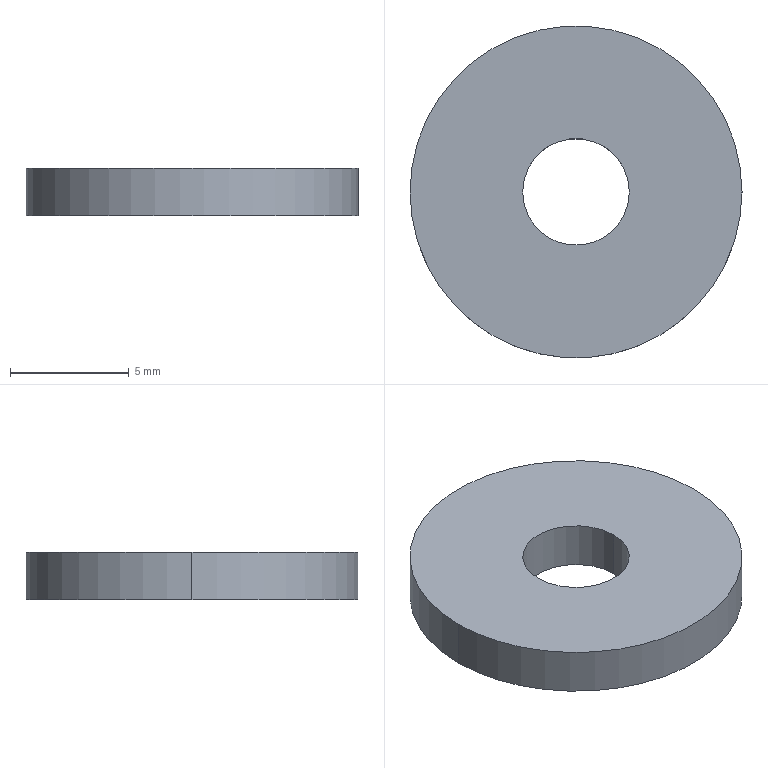Part | SolidWorks | features Extrusion 1 | 1 solid | 6 faces | box 14 x 14 x 2 mm | volume 276.067 mm3 | cylinder 4 | plane 2 | commonest cylinder face diameters 4.5 x2 14 x2
STEP:
#1=CARTESIAN_POINT('',(-2.25,0.,2.));
#2=VERTEX_POINT('',#1);
#3=CARTESIAN_POINT('',(2.25,0.,2.));
#4=VERTEX_POINT('',#3);
#5=CARTESIAN_POINT('',(0.,0.,2.));
#6=DIRECTION('',(0.,0.,1.));
#7=DIRECTION('',(1.,0.,0.));
#8=AXIS2_PLACEMENT_3D('',#5,#6,#7);
#9=CIRCLE('',#8,2.25);
#10=EDGE_CURVE('',#2,#4,#9,.T.);
#11=ORIENTED_EDGE('',*,*,#10,.T.);
#12=CARTESIAN_POINT('',(2.25,0.,0.));
#13=VERTEX_POINT('',#12);
#14=CARTESIAN_POINT('',(2.25,0.,2.));
#15=DIRECTION('',(0.,0.,-1.));
#16=VECTOR('',#15,1000.);
#17=LINE('',#14,#16);
#18=EDGE_CURVE('',#4,#13,#17,.T.);
#19=ORIENTED_EDGE('',*,*,#18,.T.);
#20=CARTESIAN_POINT('',(-2.25,0.,0.));
#21=VERTEX_POINT('',#20);
#22=CARTESIAN_POINT('',(0.,0.,0.));
#23=DIRECTION('',(0.,0.,1.));
#24=DIRECTION('',(1.,0.,0.));
#25=AXIS2_PLACEMENT_3D('',#22,#23,#24);
#26=CIRCLE('',#25,2.25);
#27=EDGE_CURVE('',#21,#13,#26,.T.);
#28=ORIENTED_EDGE('',*,*,#27,.F.);
#29=CARTESIAN_POINT('',(-2.25,0.,2.));
#30=DIRECTION('',(0.,0.,-1.));
#31=VECTOR('',#30,1000.);
#32=LINE('',#29,#31);
#33=EDGE_CURVE('',#2,#21,#32,.T.);
#34=ORIENTED_EDGE('',*,*,#33,.F.);
#35=EDGE_LOOP('',(#11,#19,#28,#34));
#36=FACE_OUTER_BOUND('',#35,.T.);
#37=CARTESIAN_POINT('',(0.,0.,2.));
#38=DIRECTION('',(0.,0.,-1.));
#39=DIRECTION('',(-1.,0.,0.));
#40=AXIS2_PLACEMENT_3D('',#37,#38,#39);
#41=CYLINDRICAL_SURFACE('',#40,2.25);
#42=ADVANCED_FACE('',(#36),#41,.F.);
#43=CARTESIAN_POINT('',(7.,0.,2.));
#44=VERTEX_POINT('',#43);
#45=CARTESIAN_POINT('',(-7.,0.,2.));
#46=VERTEX_POINT('',#45);
#47=CARTESIAN_POINT('',(0.,0.,2.));
#48=DIRECTION('',(0.,0.,1.));
#49=DIRECTION('',(1.,0.,0.));
#50=AXIS2_PLACEMENT_3D('',#47,#48,#49);
#51=CIRCLE('',#50,7.);
#52=EDGE_CURVE('',#44,#46,#51,.T.);
#53=ORIENTED_EDGE('',*,*,#52,.F.);
#54=CARTESIAN_POINT('',(7.,0.,0.));
#55=VERTEX_POINT('',#54);
#56=CARTESIAN_POINT('',(7.,0.,2.));
#57=DIRECTION('',(0.,0.,-1.));
#58=VECTOR('',#57,1000.);
#59=LINE('',#56,#58);
#60=EDGE_CURVE('',#44,#55,#59,.T.);
#61=ORIENTED_EDGE('',*,*,#60,.T.);
#62=CARTESIAN_POINT('',(-7.,0.,0.));
#63=VERTEX_POINT('',#62);
#64=CARTESIAN_POINT('',(0.,0.,0.));
#65=DIRECTION('',(0.,0.,1.));
#66=DIRECTION('',(1.,0.,0.));
#67=AXIS2_PLACEMENT_3D('',#64,#65,#66);
#68=CIRCLE('',#67,7.);
#69=EDGE_CURVE('',#55,#63,#68,.T.);
#70=ORIENTED_EDGE('',*,*,#69,.T.);
#71=CARTESIAN_POINT('',(-7.,0.,2.));
#72=DIRECTION('',(0.,0.,-1.));
#73=VECTOR('',#72,1000.);
#74=LINE('',#71,#73);
#75=EDGE_CURVE('',#46,#63,#74,.T.);
#76=ORIENTED_EDGE('',*,*,#75,.F.);
#77=EDGE_LOOP('',(#53,#61,#70,#76));
#78=FACE_OUTER_BOUND('',#77,.T.);
#79=CARTESIAN_POINT('',(0.,0.,2.));
#80=DIRECTION('',(0.,0.,-1.));
#81=DIRECTION('',(-1.,0.,0.));
#82=AXIS2_PLACEMENT_3D('',#79,#80,#81);
#83=CYLINDRICAL_SURFACE('',#82,7.);
#84=ADVANCED_FACE('',(#78),#83,.T.);
#85=CARTESIAN_POINT('',(0.,0.,2.));
#86=DIRECTION('',(0.,0.,1.));
#87=DIRECTION('',(1.,0.,0.));
#88=AXIS2_PLACEMENT_3D('',#85,#86,#87);
#89=CIRCLE('',#88,7.);
#90=EDGE_CURVE('',#46,#44,#89,.T.);
#91=ORIENTED_EDGE('',*,*,#90,.T.);
#92=ORIENTED_EDGE('',*,*,#52,.T.);
#93=EDGE_LOOP('',(#91,#92));
#94=FACE_OUTER_BOUND('',#93,.T.);
#95=ORIENTED_EDGE('',*,*,#10,.F.);
#96=CARTESIAN_POINT('',(0.,0.,2.));
#97=DIRECTION('',(0.,0.,1.));
#98=DIRECTION('',(1.,0.,0.));
#99=AXIS2_PLACEMENT_3D('',#96,#97,#98);
#100=CIRCLE('',#99,2.25);
#101=EDGE_CURVE('',#4,#2,#100,.T.);
#102=ORIENTED_EDGE('',*,*,#101,.F.);
#103=EDGE_LOOP('',(#95,#102));
#104=FACE_BOUND('',#103,.T.);
#105=CARTESIAN_POINT('',(0.,0.,2.));
#106=DIRECTION('',(0.,0.,1.));
#107=DIRECTION('',(1.,0.,0.));
#108=AXIS2_PLACEMENT_3D('',#105,#106,#107);
#109=PLANE('',#108);
#110=ADVANCED_FACE('',(#94,#104),#109,.T.);
#111=CARTESIAN_POINT('',(0.,0.,0.));
#112=DIRECTION('',(0.,0.,1.));
#113=DIRECTION('',(1.,0.,0.));
#114=AXIS2_PLACEMENT_3D('',#111,#112,#113);
#115=CIRCLE('',#114,7.);
#116=EDGE_CURVE('',#63,#55,#115,.T.);
#117=ORIENTED_EDGE('',*,*,#116,.F.);
#118=ORIENTED_EDGE('',*,*,#69,.F.);
#119=EDGE_LOOP('',(#117,#118));
#120=FACE_OUTER_BOUND('',#119,.T.);
#121=ORIENTED_EDGE('',*,*,#27,.T.);
#122=CARTESIAN_POINT('',(0.,0.,0.));
#123=DIRECTION('',(0.,0.,1.));
#124=DIRECTION('',(1.,0.,0.));
#125=AXIS2_PLACEMENT_3D('',#122,#123,#124);
#126=CIRCLE('',#125,2.25);
#127=EDGE_CURVE('',#13,#21,#126,.T.);
#128=ORIENTED_EDGE('',*,*,#127,.T.);
#129=EDGE_LOOP('',(#121,#128));
#130=FACE_BOUND('',#129,.T.);
#131=CARTESIAN_POINT('',(0.,0.,0.));
#132=DIRECTION('',(0.,0.,1.));
#133=DIRECTION('',(1.,0.,0.));
#134=AXIS2_PLACEMENT_3D('',#131,#132,#133);
#135=PLANE('',#134);
#136=ADVANCED_FACE('',(#120,#130),#135,.F.);
#137=ORIENTED_EDGE('',*,*,#60,.F.);
#138=ORIENTED_EDGE('',*,*,#90,.F.);
#139=ORIENTED_EDGE('',*,*,#75,.T.);
#140=ORIENTED_EDGE('',*,*,#116,.T.);
#141=EDGE_LOOP('',(#137,#138,#139,#140));
#142=FACE_OUTER_BOUND('',#141,.T.);
#143=CARTESIAN_POINT('',(0.,0.,2.));
#144=DIRECTION('',(0.,0.,-1.));
#145=DIRECTION('',(-1.,0.,0.));
#146=AXIS2_PLACEMENT_3D('',#143,#144,#145);
#147=CYLINDRICAL_SURFACE('',#146,7.);
#148=ADVANCED_FACE('',(#142),#147,.T.);
#149=ORIENTED_EDGE('',*,*,#18,.F.);
#150=ORIENTED_EDGE('',*,*,#101,.T.);
#151=ORIENTED_EDGE('',*,*,#33,.T.);
#152=ORIENTED_EDGE('',*,*,#127,.F.);
#153=EDGE_LOOP('',(#149,#150,#151,#152));
#154=FACE_OUTER_BOUND('',#153,.T.);
#155=CARTESIAN_POINT('',(0.,0.,2.));
#156=DIRECTION('',(0.,0.,-1.));
#157=DIRECTION('',(-1.,0.,0.));
#158=AXIS2_PLACEMENT_3D('',#155,#156,#157);
#159=CYLINDRICAL_SURFACE('',#158,2.25);
#160=ADVANCED_FACE('',(#154),#159,.F.);
#161=CLOSED_SHELL('',(#42,#84,#110,#136,#148,#160));
#162=MANIFOLD_SOLID_BREP('',#161);
#163=CARTESIAN_POINT('',(0.,0.,0.));
#164=DIRECTION('',(0.,0.,1.));
#165=DIRECTION('',(1.,0.,0.));
#166=AXIS2_PLACEMENT_3D('',#163,#164,#165);
#167=(LENGTH_UNIT()NAMED_UNIT(*)SI_UNIT(.MILLI.,.METRE.));
#168=UNCERTAINTY_MEASURE_WITH_UNIT(LENGTH_MEASURE(0.00001),#167,'','');
#169=(NAMED_UNIT(*)PLANE_ANGLE_UNIT()SI_UNIT($,.RADIAN.));
#170=(NAMED_UNIT(*)SI_UNIT($,.STERADIAN.)SOLID_ANGLE_UNIT());
#171=(GEOMETRIC_REPRESENTATION_CONTEXT(3)GLOBAL_UNCERTAINTY_ASSIGNED_CONTEXT((#168))GLOBAL_UNIT_ASSIGNED_CONTEXT((#167,#169,#170))REPRESENTATION_CONTEXT('',''));
#172=ADVANCED_BREP_SHAPE_REPRESENTATION('',(#162,#166),#171);